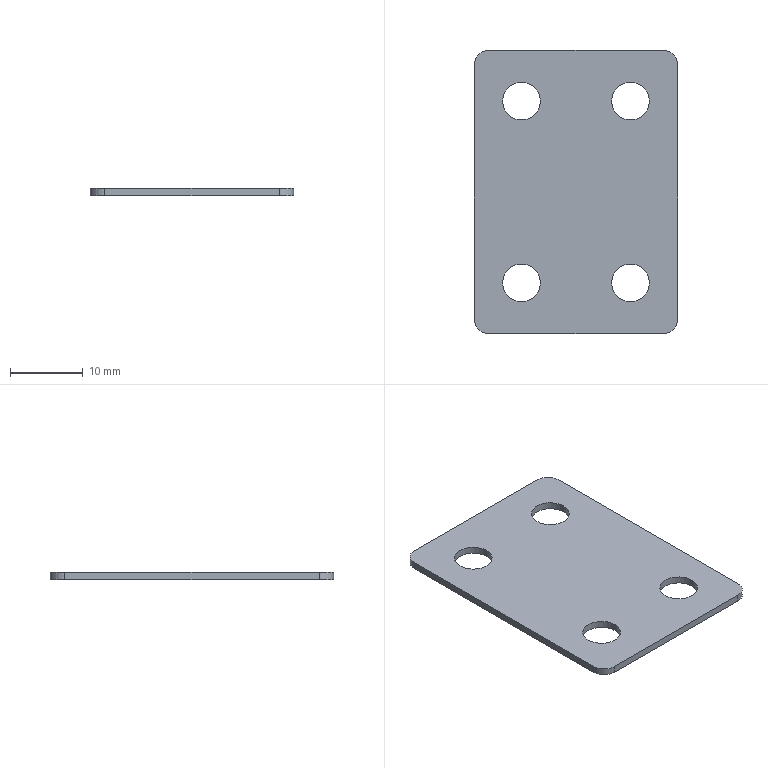Part | SolidWorks | features BaseBody 1 | 1 solid | 18 faces | box 28 x 39 x 1 mm | volume 1004 mm3 | cylinder 12 | plane 6 | commonest cylinder face diameters 5.2 x8 4 x4
STEP:
#1=CARTESIAN_POINT('',(-4.9,-12.5,1.));
#2=VERTEX_POINT('',#1);
#3=CARTESIAN_POINT('',(-10.1,-12.5,1.));
#4=VERTEX_POINT('',#3);
#5=CARTESIAN_POINT('',(-7.5,-12.5,1.));
#6=DIRECTION('',(0.,0.,-1.));
#7=DIRECTION('',(-1.,0.,0.));
#8=AXIS2_PLACEMENT_3D('',#5,#6,#7);
#9=CIRCLE('',#8,2.6);
#10=EDGE_CURVE('',#2,#4,#9,.T.);
#11=ORIENTED_EDGE('',*,*,#10,.F.);
#12=CARTESIAN_POINT('',(-4.9,-12.5,0.));
#13=VERTEX_POINT('',#12);
#14=CARTESIAN_POINT('',(-4.9,-12.5,1.));
#15=DIRECTION('',(0.,0.,-1.));
#16=VECTOR('',#15,1000.);
#17=LINE('',#14,#16);
#18=EDGE_CURVE('',#2,#13,#17,.T.);
#19=ORIENTED_EDGE('',*,*,#18,.T.);
#20=CARTESIAN_POINT('',(-10.1,-12.5,0.));
#21=VERTEX_POINT('',#20);
#22=CARTESIAN_POINT('',(-7.5,-12.5,0.));
#23=DIRECTION('',(0.,0.,1.));
#24=DIRECTION('',(-1.,0.,0.));
#25=AXIS2_PLACEMENT_3D('',#22,#23,#24);
#26=CIRCLE('',#25,2.6);
#27=EDGE_CURVE('',#21,#13,#26,.T.);
#28=ORIENTED_EDGE('',*,*,#27,.F.);
#29=CARTESIAN_POINT('',(-10.1,-12.5,1.));
#30=DIRECTION('',(0.,0.,-1.));
#31=VECTOR('',#30,1000.);
#32=LINE('',#29,#31);
#33=EDGE_CURVE('',#4,#21,#32,.T.);
#34=ORIENTED_EDGE('',*,*,#33,.F.);
#35=EDGE_LOOP('',(#11,#19,#28,#34));
#36=FACE_OUTER_BOUND('',#35,.T.);
#37=CARTESIAN_POINT('',(-7.5,-12.5,1.));
#38=DIRECTION('',(0.,0.,-1.));
#39=DIRECTION('',(-1.,0.,0.));
#40=AXIS2_PLACEMENT_3D('',#37,#38,#39);
#41=CYLINDRICAL_SURFACE('',#40,2.6);
#42=ADVANCED_FACE('',(#36),#41,.F.);
#43=CARTESIAN_POINT('',(10.1,12.5,1.));
#44=VERTEX_POINT('',#43);
#45=CARTESIAN_POINT('',(4.9,12.5,1.));
#46=VERTEX_POINT('',#45);
#47=CARTESIAN_POINT('',(7.5,12.5,1.));
#48=DIRECTION('',(0.,0.,-1.));
#49=DIRECTION('',(-1.,0.,0.));
#50=AXIS2_PLACEMENT_3D('',#47,#48,#49);
#51=CIRCLE('',#50,2.6);
#52=EDGE_CURVE('',#44,#46,#51,.T.);
#53=ORIENTED_EDGE('',*,*,#52,.F.);
#54=CARTESIAN_POINT('',(10.1,12.5,0.));
#55=VERTEX_POINT('',#54);
#56=CARTESIAN_POINT('',(10.1,12.5,1.));
#57=DIRECTION('',(0.,0.,-1.));
#58=VECTOR('',#57,1000.);
#59=LINE('',#56,#58);
#60=EDGE_CURVE('',#44,#55,#59,.T.);
#61=ORIENTED_EDGE('',*,*,#60,.T.);
#62=CARTESIAN_POINT('',(4.9,12.5,0.));
#63=VERTEX_POINT('',#62);
#64=CARTESIAN_POINT('',(7.5,12.5,0.));
#65=DIRECTION('',(0.,0.,1.));
#66=DIRECTION('',(-1.,0.,0.));
#67=AXIS2_PLACEMENT_3D('',#64,#65,#66);
#68=CIRCLE('',#67,2.6);
#69=EDGE_CURVE('',#63,#55,#68,.T.);
#70=ORIENTED_EDGE('',*,*,#69,.F.);
#71=CARTESIAN_POINT('',(4.9,12.5,1.));
#72=DIRECTION('',(0.,0.,-1.));
#73=VECTOR('',#72,1000.);
#74=LINE('',#71,#73);
#75=EDGE_CURVE('',#46,#63,#74,.T.);
#76=ORIENTED_EDGE('',*,*,#75,.F.);
#77=EDGE_LOOP('',(#53,#61,#70,#76));
#78=FACE_OUTER_BOUND('',#77,.T.);
#79=CARTESIAN_POINT('',(7.5,12.5,1.));
#80=DIRECTION('',(0.,0.,-1.));
#81=DIRECTION('',(-1.,0.,0.));
#82=AXIS2_PLACEMENT_3D('',#79,#80,#81);
#83=CYLINDRICAL_SURFACE('',#82,2.6);
#84=ADVANCED_FACE('',(#78),#83,.F.);
#85=CARTESIAN_POINT('',(-4.9,12.5,1.));
#86=VERTEX_POINT('',#85);
#87=CARTESIAN_POINT('',(-10.1,12.5,1.));
#88=VERTEX_POINT('',#87);
#89=CARTESIAN_POINT('',(-7.5,12.5,1.));
#90=DIRECTION('',(0.,0.,-1.));
#91=DIRECTION('',(-1.,0.,0.));
#92=AXIS2_PLACEMENT_3D('',#89,#90,#91);
#93=CIRCLE('',#92,2.6);
#94=EDGE_CURVE('',#86,#88,#93,.T.);
#95=ORIENTED_EDGE('',*,*,#94,.F.);
#96=CARTESIAN_POINT('',(-4.9,12.5,0.));
#97=VERTEX_POINT('',#96);
#98=CARTESIAN_POINT('',(-4.9,12.5,1.));
#99=DIRECTION('',(0.,0.,-1.));
#100=VECTOR('',#99,1000.);
#101=LINE('',#98,#100);
#102=EDGE_CURVE('',#86,#97,#101,.T.);
#103=ORIENTED_EDGE('',*,*,#102,.T.);
#104=CARTESIAN_POINT('',(-10.1,12.5,0.));
#105=VERTEX_POINT('',#104);
#106=CARTESIAN_POINT('',(-7.5,12.5,0.));
#107=DIRECTION('',(0.,0.,1.));
#108=DIRECTION('',(-1.,0.,0.));
#109=AXIS2_PLACEMENT_3D('',#106,#107,#108);
#110=CIRCLE('',#109,2.6);
#111=EDGE_CURVE('',#105,#97,#110,.T.);
#112=ORIENTED_EDGE('',*,*,#111,.F.);
#113=CARTESIAN_POINT('',(-10.1,12.5,1.));
#114=DIRECTION('',(0.,0.,-1.));
#115=VECTOR('',#114,1000.);
#116=LINE('',#113,#115);
#117=EDGE_CURVE('',#88,#105,#116,.T.);
#118=ORIENTED_EDGE('',*,*,#117,.F.);
#119=EDGE_LOOP('',(#95,#103,#112,#118));
#120=FACE_OUTER_BOUND('',#119,.T.);
#121=CARTESIAN_POINT('',(-7.5,12.5,1.));
#122=DIRECTION('',(0.,0.,-1.));
#123=DIRECTION('',(-1.,0.,0.));
#124=AXIS2_PLACEMENT_3D('',#121,#122,#123);
#125=CYLINDRICAL_SURFACE('',#124,2.6);
#126=ADVANCED_FACE('',(#120),#125,.F.);
#127=CARTESIAN_POINT('',(10.1,-12.5,1.));
#128=VERTEX_POINT('',#127);
#129=CARTESIAN_POINT('',(4.9,-12.5,1.));
#130=VERTEX_POINT('',#129);
#131=CARTESIAN_POINT('',(7.5,-12.5,1.));
#132=DIRECTION('',(0.,0.,-1.));
#133=DIRECTION('',(-1.,0.,0.));
#134=AXIS2_PLACEMENT_3D('',#131,#132,#133);
#135=CIRCLE('',#134,2.6);
#136=EDGE_CURVE('',#128,#130,#135,.T.);
#137=ORIENTED_EDGE('',*,*,#136,.F.);
#138=CARTESIAN_POINT('',(10.1,-12.5,0.));
#139=VERTEX_POINT('',#138);
#140=CARTESIAN_POINT('',(10.1,-12.5,1.));
#141=DIRECTION('',(0.,0.,-1.));
#142=VECTOR('',#141,1000.);
#143=LINE('',#140,#142);
#144=EDGE_CURVE('',#128,#139,#143,.T.);
#145=ORIENTED_EDGE('',*,*,#144,.T.);
#146=CARTESIAN_POINT('',(4.9,-12.5,0.));
#147=VERTEX_POINT('',#146);
#148=CARTESIAN_POINT('',(7.5,-12.5,0.));
#149=DIRECTION('',(0.,0.,1.));
#150=DIRECTION('',(-1.,0.,0.));
#151=AXIS2_PLACEMENT_3D('',#148,#149,#150);
#152=CIRCLE('',#151,2.6);
#153=EDGE_CURVE('',#147,#139,#152,.T.);
#154=ORIENTED_EDGE('',*,*,#153,.F.);
#155=CARTESIAN_POINT('',(4.9,-12.5,1.));
#156=DIRECTION('',(0.,0.,-1.));
#157=VECTOR('',#156,1000.);
#158=LINE('',#155,#157);
#159=EDGE_CURVE('',#130,#147,#158,.T.);
#160=ORIENTED_EDGE('',*,*,#159,.F.);
#161=EDGE_LOOP('',(#137,#145,#154,#160));
#162=FACE_OUTER_BOUND('',#161,.T.);
#163=CARTESIAN_POINT('',(7.5,-12.5,1.));
#164=DIRECTION('',(0.,0.,-1.));
#165=DIRECTION('',(-1.,0.,0.));
#166=AXIS2_PLACEMENT_3D('',#163,#164,#165);
#167=CYLINDRICAL_SURFACE('',#166,2.6);
#168=ADVANCED_FACE('',(#162),#167,.F.);
#169=CARTESIAN_POINT('',(-7.5,-12.5,1.));
#170=DIRECTION('',(0.,0.,-1.));
#171=DIRECTION('',(-1.,0.,0.));
#172=AXIS2_PLACEMENT_3D('',#169,#170,#171);
#173=CIRCLE('',#172,2.6);
#174=EDGE_CURVE('',#4,#2,#173,.T.);
#175=ORIENTED_EDGE('',*,*,#174,.T.);
#176=ORIENTED_EDGE('',*,*,#10,.T.);
#177=EDGE_LOOP('',(#175,#176));
#178=FACE_BOUND('',#177,.T.);
#179=CARTESIAN_POINT('',(7.5,12.5,1.));
#180=DIRECTION('',(0.,0.,-1.));
#181=DIRECTION('',(-1.,0.,0.));
#182=AXIS2_PLACEMENT_3D('',#179,#180,#181);
#183=CIRCLE('',#182,2.6);
#184=EDGE_CURVE('',#46,#44,#183,.T.);
#185=ORIENTED_EDGE('',*,*,#184,.T.);
#186=ORIENTED_EDGE('',*,*,#52,.T.);
#187=EDGE_LOOP('',(#185,#186));
#188=FACE_BOUND('',#187,.T.);
#189=CARTESIAN_POINT('',(12.,19.5,1.));
#190=VERTEX_POINT('',#189);
#191=CARTESIAN_POINT('',(-12.,19.5,1.));
#192=VERTEX_POINT('',#191);
#193=CARTESIAN_POINT('',(0.,19.5,1.));
#194=DIRECTION('',(-1.,0.,0.));
#195=VECTOR('',#194,1000.);
#196=LINE('',#193,#195);
#197=EDGE_CURVE('',#190,#192,#196,.T.);
#198=ORIENTED_EDGE('',*,*,#197,.T.);
#199=CARTESIAN_POINT('',(-14.,17.5,1.));
#200=VERTEX_POINT('',#199);
#201=CARTESIAN_POINT('',(-12.,17.5,1.));
#202=DIRECTION('',(0.,0.,1.));
#203=DIRECTION('',(-1.,0.,0.));
#204=AXIS2_PLACEMENT_3D('',#201,#202,#203);
#205=CIRCLE('',#204,2.);
#206=EDGE_CURVE('',#192,#200,#205,.T.);
#207=ORIENTED_EDGE('',*,*,#206,.T.);
#208=CARTESIAN_POINT('',(-14.,-17.5,1.));
#209=VERTEX_POINT('',#208);
#210=CARTESIAN_POINT('',(-14.,0.,1.));
#211=DIRECTION('',(0.,-1.,0.));
#212=VECTOR('',#211,1000.);
#213=LINE('',#210,#212);
#214=EDGE_CURVE('',#200,#209,#213,.T.);
#215=ORIENTED_EDGE('',*,*,#214,.T.);
#216=CARTESIAN_POINT('',(-12.,-19.5,1.));
#217=VERTEX_POINT('',#216);
#218=CARTESIAN_POINT('',(-12.,-17.5,1.));
#219=DIRECTION('',(0.,0.,1.));
#220=DIRECTION('',(-1.,0.,0.));
#221=AXIS2_PLACEMENT_3D('',#218,#219,#220);
#222=CIRCLE('',#221,2.);
#223=EDGE_CURVE('',#209,#217,#222,.T.);
#224=ORIENTED_EDGE('',*,*,#223,.T.);
#225=CARTESIAN_POINT('',(12.,-19.5,1.));
#226=VERTEX_POINT('',#225);
#227=CARTESIAN_POINT('',(0.,-19.5,1.));
#228=DIRECTION('',(1.,0.,0.));
#229=VECTOR('',#228,1000.);
#230=LINE('',#227,#229);
#231=EDGE_CURVE('',#217,#226,#230,.T.);
#232=ORIENTED_EDGE('',*,*,#231,.T.);
#233=CARTESIAN_POINT('',(14.,-17.5,1.));
#234=VERTEX_POINT('',#233);
#235=CARTESIAN_POINT('',(12.,-17.5,1.));
#236=DIRECTION('',(0.,0.,1.));
#237=DIRECTION('',(-1.,0.,0.));
#238=AXIS2_PLACEMENT_3D('',#235,#236,#237);
#239=CIRCLE('',#238,2.);
#240=EDGE_CURVE('',#226,#234,#239,.T.);
#241=ORIENTED_EDGE('',*,*,#240,.T.);
#242=CARTESIAN_POINT('',(14.,17.5,1.));
#243=VERTEX_POINT('',#242);
#244=CARTESIAN_POINT('',(14.,0.,1.));
#245=DIRECTION('',(0.,1.,0.));
#246=VECTOR('',#245,1000.);
#247=LINE('',#244,#246);
#248=EDGE_CURVE('',#234,#243,#247,.T.);
#249=ORIENTED_EDGE('',*,*,#248,.T.);
#250=CARTESIAN_POINT('',(12.,17.5,1.));
#251=DIRECTION('',(0.,0.,1.));
#252=DIRECTION('',(-1.,0.,0.));
#253=AXIS2_PLACEMENT_3D('',#250,#251,#252);
#254=CIRCLE('',#253,2.);
#255=EDGE_CURVE('',#243,#190,#254,.T.);
#256=ORIENTED_EDGE('',*,*,#255,.T.);
#257=EDGE_LOOP('',(#198,#207,#215,#224,#232,#241,#249,#256));
#258=FACE_OUTER_BOUND('',#257,.T.);
#259=CARTESIAN_POINT('',(-7.5,12.5,1.));
#260=DIRECTION('',(0.,0.,-1.));
#261=DIRECTION('',(-1.,0.,0.));
#262=AXIS2_PLACEMENT_3D('',#259,#260,#261);
#263=CIRCLE('',#262,2.6);
#264=EDGE_CURVE('',#88,#86,#263,.T.);
#265=ORIENTED_EDGE('',*,*,#264,.T.);
#266=ORIENTED_EDGE('',*,*,#94,.T.);
#267=EDGE_LOOP('',(#265,#266));
#268=FACE_BOUND('',#267,.T.);
#269=CARTESIAN_POINT('',(7.5,-12.5,1.));
#270=DIRECTION('',(0.,0.,-1.));
#271=DIRECTION('',(-1.,0.,0.));
#272=AXIS2_PLACEMENT_3D('',#269,#270,#271);
#273=CIRCLE('',#272,2.6);
#274=EDGE_CURVE('',#130,#128,#273,.T.);
#275=ORIENTED_EDGE('',*,*,#274,.T.);
#276=ORIENTED_EDGE('',*,*,#136,.T.);
#277=EDGE_LOOP('',(#275,#276));
#278=FACE_BOUND('',#277,.T.);
#279=CARTESIAN_POINT('',(0.,0.,1.));
#280=DIRECTION('',(0.,0.,1.));
#281=DIRECTION('',(1.,0.,0.));
#282=AXIS2_PLACEMENT_3D('',#279,#280,#281);
#283=PLANE('',#282);
#284=ADVANCED_FACE('',(#178,#188,#258,#268,#278),#283,.T.);
#285=ORIENTED_EDGE('',*,*,#18,.F.);
#286=ORIENTED_EDGE('',*,*,#174,.F.);
#287=ORIENTED_EDGE('',*,*,#33,.T.);
#288=CARTESIAN_POINT('',(-7.5,-12.5,0.));
#289=DIRECTION('',(0.,0.,1.));
#290=DIRECTION('',(-1.,0.,0.));
#291=AXIS2_PLACEMENT_3D('',#288,#289,#290);
#292=CIRCLE('',#291,2.6);
#293=EDGE_CURVE('',#13,#21,#292,.T.);
#294=ORIENTED_EDGE('',*,*,#293,.F.);
#295=EDGE_LOOP('',(#285,#286,#287,#294));
#296=FACE_OUTER_BOUND('',#295,.T.);
#297=CARTESIAN_POINT('',(-7.5,-12.5,1.));
#298=DIRECTION('',(0.,0.,-1.));
#299=DIRECTION('',(-1.,0.,0.));
#300=AXIS2_PLACEMENT_3D('',#297,#298,#299);
#301=CYLINDRICAL_SURFACE('',#300,2.6);
#302=ADVANCED_FACE('',(#296),#301,.F.);
#303=ORIENTED_EDGE('',*,*,#60,.F.);
#304=ORIENTED_EDGE('',*,*,#184,.F.);
#305=ORIENTED_EDGE('',*,*,#75,.T.);
#306=CARTESIAN_POINT('',(7.5,12.5,0.));
#307=DIRECTION('',(0.,0.,1.));
#308=DIRECTION('',(-1.,0.,0.));
#309=AXIS2_PLACEMENT_3D('',#306,#307,#308);
#310=CIRCLE('',#309,2.6);
#311=EDGE_CURVE('',#55,#63,#310,.T.);
#312=ORIENTED_EDGE('',*,*,#311,.F.);
#313=EDGE_LOOP('',(#303,#304,#305,#312));
#314=FACE_OUTER_BOUND('',#313,.T.);
#315=CARTESIAN_POINT('',(7.5,12.5,1.));
#316=DIRECTION('',(0.,0.,-1.));
#317=DIRECTION('',(-1.,0.,0.));
#318=AXIS2_PLACEMENT_3D('',#315,#316,#317);
#319=CYLINDRICAL_SURFACE('',#318,2.6);
#320=ADVANCED_FACE('',(#314),#319,.F.);
#321=CARTESIAN_POINT('',(-12.,19.5,0.));
#322=VERTEX_POINT('',#321);
#323=CARTESIAN_POINT('',(-14.,17.5,0.));
#324=VERTEX_POINT('',#323);
#325=CARTESIAN_POINT('',(-12.,17.5,0.));
#326=DIRECTION('',(0.,0.,1.));
#327=DIRECTION('',(-1.,0.,0.));
#328=AXIS2_PLACEMENT_3D('',#325,#326,#327);
#329=CIRCLE('',#328,2.);
#330=EDGE_CURVE('',#322,#324,#329,.T.);
#331=ORIENTED_EDGE('',*,*,#330,.T.);
#332=CARTESIAN_POINT('',(-14.,17.5,1.));
#333=DIRECTION('',(0.,0.,1.));
#334=VECTOR('',#333,1000.);
#335=LINE('',#332,#334);
#336=EDGE_CURVE('',#324,#200,#335,.T.);
#337=ORIENTED_EDGE('',*,*,#336,.T.);
#338=ORIENTED_EDGE('',*,*,#206,.F.);
#339=CARTESIAN_POINT('',(-12.,19.5,1.));
#340=DIRECTION('',(0.,0.,-1.));
#341=VECTOR('',#340,1000.);
#342=LINE('',#339,#341);
#343=EDGE_CURVE('',#192,#322,#342,.T.);
#344=ORIENTED_EDGE('',*,*,#343,.T.);
#345=EDGE_LOOP('',(#331,#337,#338,#344));
#346=FACE_OUTER_BOUND('',#345,.T.);
#347=CARTESIAN_POINT('',(-12.,17.5,1.));
#348=DIRECTION('',(0.,0.,-1.));
#349=DIRECTION('',(-1.,0.,0.));
#350=AXIS2_PLACEMENT_3D('',#347,#348,#349);
#351=CYLINDRICAL_SURFACE('',#350,2.);
#352=ADVANCED_FACE('',(#346),#351,.T.);
#353=CARTESIAN_POINT('',(12.,19.5,0.));
#354=VERTEX_POINT('',#353);
#355=CARTESIAN_POINT('',(12.,19.5,1.));
#356=DIRECTION('',(0.,0.,1.));
#357=VECTOR('',#356,1000.);
#358=LINE('',#355,#357);
#359=EDGE_CURVE('',#354,#190,#358,.T.);
#360=ORIENTED_EDGE('',*,*,#359,.F.);
#361=CARTESIAN_POINT('',(14.,19.5,0.));
#362=DIRECTION('',(1.,0.,0.));
#363=VECTOR('',#362,1000.);
#364=LINE('',#361,#363);
#365=EDGE_CURVE('',#322,#354,#364,.T.);
#366=ORIENTED_EDGE('',*,*,#365,.F.);
#367=ORIENTED_EDGE('',*,*,#343,.F.);
#368=ORIENTED_EDGE('',*,*,#197,.F.);
#369=EDGE_LOOP('',(#360,#366,#367,#368));
#370=FACE_OUTER_BOUND('',#369,.T.);
#371=CARTESIAN_POINT('',(14.,19.5,1.));
#372=DIRECTION('',(0.,-1.,0.));
#373=DIRECTION('',(0.,0.,-1.));
#374=AXIS2_PLACEMENT_3D('',#371,#372,#373);
#375=PLANE('',#374);
#376=ADVANCED_FACE('',(#370),#375,.F.);
#377=CARTESIAN_POINT('',(14.,17.5,0.));
#378=VERTEX_POINT('',#377);
#379=CARTESIAN_POINT('',(12.,17.5,0.));
#380=DIRECTION('',(0.,0.,1.));
#381=DIRECTION('',(-1.,0.,0.));
#382=AXIS2_PLACEMENT_3D('',#379,#380,#381);
#383=CIRCLE('',#382,2.);
#384=EDGE_CURVE('',#378,#354,#383,.T.);
#385=ORIENTED_EDGE('',*,*,#384,.T.);
#386=ORIENTED_EDGE('',*,*,#359,.T.);
#387=ORIENTED_EDGE('',*,*,#255,.F.);
#388=CARTESIAN_POINT('',(14.,17.5,1.));
#389=DIRECTION('',(0.,0.,-1.));
#390=VECTOR('',#389,1000.);
#391=LINE('',#388,#390);
#392=EDGE_CURVE('',#243,#378,#391,.T.);
#393=ORIENTED_EDGE('',*,*,#392,.T.);
#394=EDGE_LOOP('',(#385,#386,#387,#393));
#395=FACE_OUTER_BOUND('',#394,.T.);
#396=CARTESIAN_POINT('',(12.,17.5,1.));
#397=DIRECTION('',(0.,0.,-1.));
#398=DIRECTION('',(-1.,0.,0.));
#399=AXIS2_PLACEMENT_3D('',#396,#397,#398);
#400=CYLINDRICAL_SURFACE('',#399,2.);
#401=ADVANCED_FACE('',(#395),#400,.T.);
#402=CARTESIAN_POINT('',(14.,-17.5,0.));
#403=VERTEX_POINT('',#402);
#404=CARTESIAN_POINT('',(14.,-17.5,1.));
#405=DIRECTION('',(0.,0.,1.));
#406=VECTOR('',#405,1000.);
#407=LINE('',#404,#406);
#408=EDGE_CURVE('',#403,#234,#407,.T.);
#409=ORIENTED_EDGE('',*,*,#408,.F.);
#410=CARTESIAN_POINT('',(14.,-19.5,0.));
#411=DIRECTION('',(0.,-1.,0.));
#412=VECTOR('',#411,1000.);
#413=LINE('',#410,#412);
#414=EDGE_CURVE('',#378,#403,#413,.T.);
#415=ORIENTED_EDGE('',*,*,#414,.F.);
#416=ORIENTED_EDGE('',*,*,#392,.F.);
#417=ORIENTED_EDGE('',*,*,#248,.F.);
#418=EDGE_LOOP('',(#409,#415,#416,#417));
#419=FACE_OUTER_BOUND('',#418,.T.);
#420=CARTESIAN_POINT('',(14.,-19.5,1.));
#421=DIRECTION('',(-1.,0.,0.));
#422=DIRECTION('',(0.,0.,1.));
#423=AXIS2_PLACEMENT_3D('',#420,#421,#422);
#424=PLANE('',#423);
#425=ADVANCED_FACE('',(#419),#424,.F.);
#426=CARTESIAN_POINT('',(12.,-19.5,0.));
#427=VERTEX_POINT('',#426);
#428=CARTESIAN_POINT('',(12.,-17.5,0.));
#429=DIRECTION('',(0.,0.,1.));
#430=DIRECTION('',(-1.,0.,0.));
#431=AXIS2_PLACEMENT_3D('',#428,#429,#430);
#432=CIRCLE('',#431,2.);
#433=EDGE_CURVE('',#427,#403,#432,.T.);
#434=ORIENTED_EDGE('',*,*,#433,.T.);
#435=ORIENTED_EDGE('',*,*,#408,.T.);
#436=ORIENTED_EDGE('',*,*,#240,.F.);
#437=CARTESIAN_POINT('',(12.,-19.5,1.));
#438=DIRECTION('',(0.,0.,-1.));
#439=VECTOR('',#438,1000.);
#440=LINE('',#437,#439);
#441=EDGE_CURVE('',#226,#427,#440,.T.);
#442=ORIENTED_EDGE('',*,*,#441,.T.);
#443=EDGE_LOOP('',(#434,#435,#436,#442));
#444=FACE_OUTER_BOUND('',#443,.T.);
#445=CARTESIAN_POINT('',(12.,-17.5,1.));
#446=DIRECTION('',(0.,0.,-1.));
#447=DIRECTION('',(-1.,0.,0.));
#448=AXIS2_PLACEMENT_3D('',#445,#446,#447);
#449=CYLINDRICAL_SURFACE('',#448,2.);
#450=ADVANCED_FACE('',(#444),#449,.T.);
#451=CARTESIAN_POINT('',(-12.,-19.5,0.));
#452=VERTEX_POINT('',#451);
#453=CARTESIAN_POINT('',(-12.,-19.5,1.));
#454=DIRECTION('',(0.,0.,1.));
#455=VECTOR('',#454,1000.);
#456=LINE('',#453,#455);
#457=EDGE_CURVE('',#452,#217,#456,.T.);
#458=ORIENTED_EDGE('',*,*,#457,.F.);
#459=CARTESIAN_POINT('',(14.,-19.5,0.));
#460=DIRECTION('',(-1.,0.,0.));
#461=VECTOR('',#460,1000.);
#462=LINE('',#459,#461);
#463=EDGE_CURVE('',#427,#452,#462,.T.);
#464=ORIENTED_EDGE('',*,*,#463,.F.);
#465=ORIENTED_EDGE('',*,*,#441,.F.);
#466=ORIENTED_EDGE('',*,*,#231,.F.);
#467=EDGE_LOOP('',(#458,#464,#465,#466));
#468=FACE_OUTER_BOUND('',#467,.T.);
#469=CARTESIAN_POINT('',(14.,-19.5,1.));
#470=DIRECTION('',(0.,1.,0.));
#471=DIRECTION('',(-1.,0.,0.));
#472=AXIS2_PLACEMENT_3D('',#469,#470,#471);
#473=PLANE('',#472);
#474=ADVANCED_FACE('',(#468),#473,.F.);
#475=CARTESIAN_POINT('',(-14.,-17.5,0.));
#476=VERTEX_POINT('',#475);
#477=CARTESIAN_POINT('',(-12.,-17.5,0.));
#478=DIRECTION('',(0.,0.,1.));
#479=DIRECTION('',(-1.,0.,0.));
#480=AXIS2_PLACEMENT_3D('',#477,#478,#479);
#481=CIRCLE('',#480,2.);
#482=EDGE_CURVE('',#476,#452,#481,.T.);
#483=ORIENTED_EDGE('',*,*,#482,.T.);
#484=ORIENTED_EDGE('',*,*,#457,.T.);
#485=ORIENTED_EDGE('',*,*,#223,.F.);
#486=CARTESIAN_POINT('',(-14.,-17.5,1.));
#487=DIRECTION('',(0.,0.,-1.));
#488=VECTOR('',#487,1000.);
#489=LINE('',#486,#488);
#490=EDGE_CURVE('',#209,#476,#489,.T.);
#491=ORIENTED_EDGE('',*,*,#490,.T.);
#492=EDGE_LOOP('',(#483,#484,#485,#491));
#493=FACE_OUTER_BOUND('',#492,.T.);
#494=CARTESIAN_POINT('',(-12.,-17.5,1.));
#495=DIRECTION('',(0.,0.,-1.));
#496=DIRECTION('',(-1.,0.,0.));
#497=AXIS2_PLACEMENT_3D('',#494,#495,#496);
#498=CYLINDRICAL_SURFACE('',#497,2.);
#499=ADVANCED_FACE('',(#493),#498,.T.);
#500=ORIENTED_EDGE('',*,*,#490,.F.);
#501=ORIENTED_EDGE('',*,*,#214,.F.);
#502=ORIENTED_EDGE('',*,*,#336,.F.);
#503=CARTESIAN_POINT('',(-14.,-19.5,0.));
#504=DIRECTION('',(0.,1.,0.));
#505=VECTOR('',#504,1000.);
#506=LINE('',#503,#505);
#507=EDGE_CURVE('',#476,#324,#506,.T.);
#508=ORIENTED_EDGE('',*,*,#507,.F.);
#509=EDGE_LOOP('',(#500,#501,#502,#508));
#510=FACE_OUTER_BOUND('',#509,.T.);
#511=CARTESIAN_POINT('',(-14.,-19.5,1.));
#512=DIRECTION('',(1.,0.,0.));
#513=DIRECTION('',(0.,1.,0.));
#514=AXIS2_PLACEMENT_3D('',#511,#512,#513);
#515=PLANE('',#514);
#516=ADVANCED_FACE('',(#510),#515,.F.);
#517=ORIENTED_EDGE('',*,*,#102,.F.);
#518=ORIENTED_EDGE('',*,*,#264,.F.);
#519=ORIENTED_EDGE('',*,*,#117,.T.);
#520=CARTESIAN_POINT('',(-7.5,12.5,0.));
#521=DIRECTION('',(0.,0.,1.));
#522=DIRECTION('',(-1.,0.,0.));
#523=AXIS2_PLACEMENT_3D('',#520,#521,#522);
#524=CIRCLE('',#523,2.6);
#525=EDGE_CURVE('',#97,#105,#524,.T.);
#526=ORIENTED_EDGE('',*,*,#525,.F.);
#527=EDGE_LOOP('',(#517,#518,#519,#526));
#528=FACE_OUTER_BOUND('',#527,.T.);
#529=CARTESIAN_POINT('',(-7.5,12.5,1.));
#530=DIRECTION('',(0.,0.,-1.));
#531=DIRECTION('',(-1.,0.,0.));
#532=AXIS2_PLACEMENT_3D('',#529,#530,#531);
#533=CYLINDRICAL_SURFACE('',#532,2.6);
#534=ADVANCED_FACE('',(#528),#533,.F.);
#535=ORIENTED_EDGE('',*,*,#144,.F.);
#536=ORIENTED_EDGE('',*,*,#274,.F.);
#537=ORIENTED_EDGE('',*,*,#159,.T.);
#538=CARTESIAN_POINT('',(7.5,-12.5,0.));
#539=DIRECTION('',(0.,0.,1.));
#540=DIRECTION('',(-1.,0.,0.));
#541=AXIS2_PLACEMENT_3D('',#538,#539,#540);
#542=CIRCLE('',#541,2.6);
#543=EDGE_CURVE('',#139,#147,#542,.T.);
#544=ORIENTED_EDGE('',*,*,#543,.F.);
#545=EDGE_LOOP('',(#535,#536,#537,#544));
#546=FACE_OUTER_BOUND('',#545,.T.);
#547=CARTESIAN_POINT('',(7.5,-12.5,1.));
#548=DIRECTION('',(0.,0.,-1.));
#549=DIRECTION('',(-1.,0.,0.));
#550=AXIS2_PLACEMENT_3D('',#547,#548,#549);
#551=CYLINDRICAL_SURFACE('',#550,2.6);
#552=ADVANCED_FACE('',(#546),#551,.F.);
#553=ORIENTED_EDGE('',*,*,#27,.T.);
#554=ORIENTED_EDGE('',*,*,#293,.T.);
#555=EDGE_LOOP('',(#553,#554));
#556=FACE_BOUND('',#555,.T.);
#557=ORIENTED_EDGE('',*,*,#153,.T.);
#558=ORIENTED_EDGE('',*,*,#543,.T.);
#559=EDGE_LOOP('',(#557,#558));
#560=FACE_BOUND('',#559,.T.);
#561=ORIENTED_EDGE('',*,*,#69,.T.);
#562=ORIENTED_EDGE('',*,*,#311,.T.);
#563=EDGE_LOOP('',(#561,#562));
#564=FACE_BOUND('',#563,.T.);
#565=ORIENTED_EDGE('',*,*,#111,.T.);
#566=ORIENTED_EDGE('',*,*,#525,.T.);
#567=EDGE_LOOP('',(#565,#566));
#568=FACE_BOUND('',#567,.T.);
#569=ORIENTED_EDGE('',*,*,#482,.F.);
#570=ORIENTED_EDGE('',*,*,#507,.T.);
#571=ORIENTED_EDGE('',*,*,#330,.F.);
#572=ORIENTED_EDGE('',*,*,#365,.T.);
#573=ORIENTED_EDGE('',*,*,#384,.F.);
#574=ORIENTED_EDGE('',*,*,#414,.T.);
#575=ORIENTED_EDGE('',*,*,#433,.F.);
#576=ORIENTED_EDGE('',*,*,#463,.T.);
#577=EDGE_LOOP('',(#569,#570,#571,#572,#573,#574,#575,#576));
#578=FACE_OUTER_BOUND('',#577,.T.);
#579=CARTESIAN_POINT('',(0.,0.,0.));
#580=DIRECTION('',(0.,0.,1.));
#581=DIRECTION('',(1.,0.,0.));
#582=AXIS2_PLACEMENT_3D('',#579,#580,#581);
#583=PLANE('',#582);
#584=ADVANCED_FACE('',(#556,#560,#564,#568,#578),#583,.F.);
#585=CLOSED_SHELL('',(#42,#84,#126,#168,#284,#302,#320,#352,#376,#401,#425,#450,#474,#499,#516,#534,#552,#584));
#586=MANIFOLD_SOLID_BREP('',#585);
#587=CARTESIAN_POINT('',(0.,0.,0.));
#588=DIRECTION('',(0.,0.,1.));
#589=DIRECTION('',(1.,0.,0.));
#590=AXIS2_PLACEMENT_3D('',#587,#588,#589);
#591=(LENGTH_UNIT()NAMED_UNIT(*)SI_UNIT(.MILLI.,.METRE.));
#592=UNCERTAINTY_MEASURE_WITH_UNIT(LENGTH_MEASURE(0.00001),#591,'','');
#593=(NAMED_UNIT(*)PLANE_ANGLE_UNIT()SI_UNIT($,.RADIAN.));
#594=(NAMED_UNIT(*)SI_UNIT($,.STERADIAN.)SOLID_ANGLE_UNIT());
#595=(GEOMETRIC_REPRESENTATION_CONTEXT(3)GLOBAL_UNCERTAINTY_ASSIGNED_CONTEXT((#592))GLOBAL_UNIT_ASSIGNED_CONTEXT((#591,#593,#594))REPRESENTATION_CONTEXT('',''));
#596=ADVANCED_BREP_SHAPE_REPRESENTATION('',(#586,#590),#595);